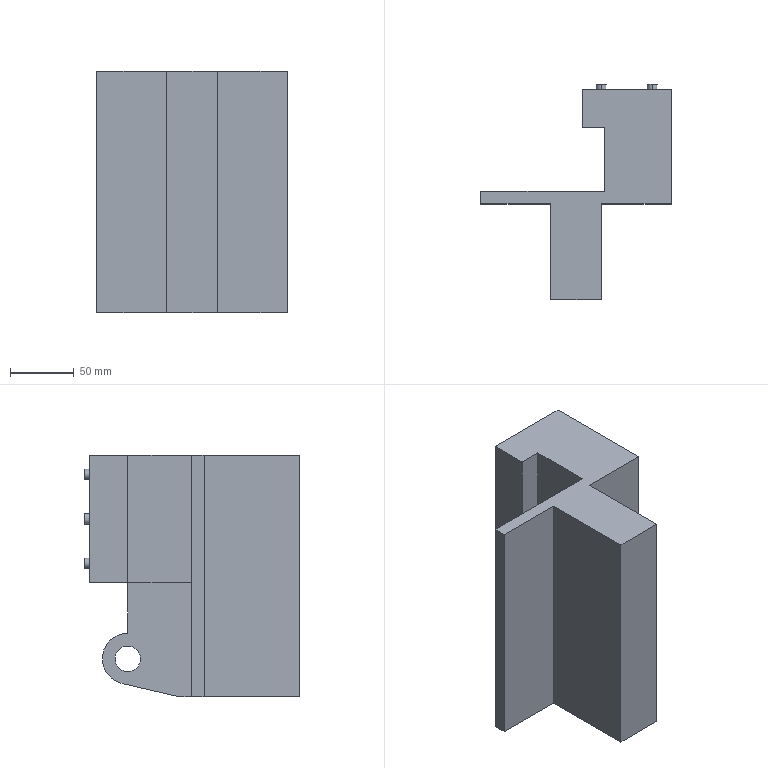Part | SolidWorks | features ICE 7, Extrusion 1, MirrorSolid 1 | 1 solid | 61 faces | box 150 x 169 x 189.781 mm | volume 1407885 mm3 | plane 50 | cylinder 11 | commonest cylinder face diameters 8 x8 20 x2 40 x1